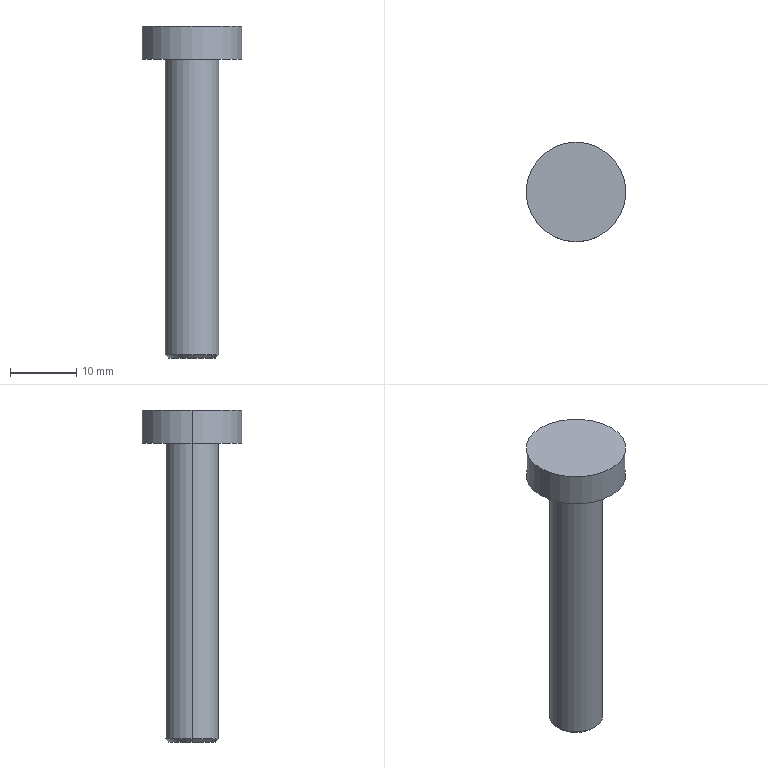Part | SolidWorks | features Chamfer 1, Extrusion 1, ICE 1 | 1 solid | 9 faces | box 15 x 15 x 50 mm | volume 3143 mm3 | cylinder 4 | plane 3 | cone 2 | commonest cylinder face diameters 8 x2 15 x2
STEP:
#1=CARTESIAN_POINT('',(-3.5,0.,0.));
#2=VERTEX_POINT('',#1);
#3=CARTESIAN_POINT('',(3.5,0.,0.));
#4=VERTEX_POINT('',#3);
#5=CARTESIAN_POINT('',(0.,0.,0.));
#6=DIRECTION('',(0.,0.,-1.));
#7=DIRECTION('',(1.,0.,0.));
#8=AXIS2_PLACEMENT_3D('',#5,#6,#7);
#9=CIRCLE('',#8,3.5);
#10=EDGE_CURVE('',#2,#4,#9,.T.);
#11=ORIENTED_EDGE('',*,*,#10,.F.);
#12=CARTESIAN_POINT('',(-4.,0.,0.5));
#13=VERTEX_POINT('',#12);
#14=CARTESIAN_POINT('',(-4.,0.,0.5));
#15=DIRECTION('',(-0.7071,0.,0.7071));
#16=VECTOR('',#15,1000.);
#17=LINE('',#14,#16);
#18=EDGE_CURVE('',#2,#13,#17,.T.);
#19=ORIENTED_EDGE('',*,*,#18,.T.);
#20=CARTESIAN_POINT('',(4.,0.,0.5));
#21=VERTEX_POINT('',#20);
#22=CARTESIAN_POINT('',(0.,0.,0.5));
#23=DIRECTION('',(0.,0.,1.));
#24=DIRECTION('',(1.,0.,0.));
#25=AXIS2_PLACEMENT_3D('',#22,#23,#24);
#26=CIRCLE('',#25,4.);
#27=EDGE_CURVE('',#21,#13,#26,.T.);
#28=ORIENTED_EDGE('',*,*,#27,.F.);
#29=CARTESIAN_POINT('',(4.,0.,0.5));
#30=DIRECTION('',(0.7071,0.,0.7071));
#31=VECTOR('',#30,1000.);
#32=LINE('',#29,#31);
#33=EDGE_CURVE('',#4,#21,#32,.T.);
#34=ORIENTED_EDGE('',*,*,#33,.F.);
#35=EDGE_LOOP('',(#11,#19,#28,#34));
#36=FACE_OUTER_BOUND('',#35,.T.);
#37=CARTESIAN_POINT('',(0.,0.,0.5));
#38=DIRECTION('',(0.,0.,1.));
#39=DIRECTION('',(1.,0.,0.));
#40=AXIS2_PLACEMENT_3D('',#37,#38,#39);
#41=CONICAL_SURFACE('',#40,4.,0.7854);
#42=ADVANCED_FACE('',(#36),#41,.T.);
#43=CARTESIAN_POINT('',(7.5,0.,50.));
#44=VERTEX_POINT('',#43);
#45=CARTESIAN_POINT('',(-7.5,0.,50.));
#46=VERTEX_POINT('',#45);
#47=CARTESIAN_POINT('',(0.,0.,50.));
#48=DIRECTION('',(0.,0.,1.));
#49=DIRECTION('',(1.,0.,0.));
#50=AXIS2_PLACEMENT_3D('',#47,#48,#49);
#51=CIRCLE('',#50,7.5);
#52=EDGE_CURVE('',#44,#46,#51,.T.);
#53=ORIENTED_EDGE('',*,*,#52,.F.);
#54=CARTESIAN_POINT('',(7.5,0.,45.));
#55=VERTEX_POINT('',#54);
#56=CARTESIAN_POINT('',(7.5,0.,50.));
#57=DIRECTION('',(0.,0.,-1.));
#58=VECTOR('',#57,1000.);
#59=LINE('',#56,#58);
#60=EDGE_CURVE('',#44,#55,#59,.T.);
#61=ORIENTED_EDGE('',*,*,#60,.T.);
#62=CARTESIAN_POINT('',(-7.5,0.,45.));
#63=VERTEX_POINT('',#62);
#64=CARTESIAN_POINT('',(0.,0.,45.));
#65=DIRECTION('',(0.,0.,1.));
#66=DIRECTION('',(1.,0.,0.));
#67=AXIS2_PLACEMENT_3D('',#64,#65,#66);
#68=CIRCLE('',#67,7.5);
#69=EDGE_CURVE('',#55,#63,#68,.T.);
#70=ORIENTED_EDGE('',*,*,#69,.T.);
#71=CARTESIAN_POINT('',(-7.5,0.,50.));
#72=DIRECTION('',(0.,0.,-1.));
#73=VECTOR('',#72,1000.);
#74=LINE('',#71,#73);
#75=EDGE_CURVE('',#46,#63,#74,.T.);
#76=ORIENTED_EDGE('',*,*,#75,.F.);
#77=EDGE_LOOP('',(#53,#61,#70,#76));
#78=FACE_OUTER_BOUND('',#77,.T.);
#79=CARTESIAN_POINT('',(0.,0.,50.));
#80=DIRECTION('',(0.,0.,-1.));
#81=DIRECTION('',(-1.,0.,0.));
#82=AXIS2_PLACEMENT_3D('',#79,#80,#81);
#83=CYLINDRICAL_SURFACE('',#82,7.5);
#84=ADVANCED_FACE('',(#78),#83,.T.);
#85=CARTESIAN_POINT('',(4.,0.,45.));
#86=VERTEX_POINT('',#85);
#87=CARTESIAN_POINT('',(-4.,0.,45.));
#88=VERTEX_POINT('',#87);
#89=CARTESIAN_POINT('',(0.,0.,45.));
#90=DIRECTION('',(0.,0.,1.));
#91=DIRECTION('',(1.,0.,0.));
#92=AXIS2_PLACEMENT_3D('',#89,#90,#91);
#93=CIRCLE('',#92,4.);
#94=EDGE_CURVE('',#86,#88,#93,.T.);
#95=ORIENTED_EDGE('',*,*,#94,.F.);
#96=CARTESIAN_POINT('',(4.,0.,45.));
#97=DIRECTION('',(0.,0.,-1.));
#98=VECTOR('',#97,1000.);
#99=LINE('',#96,#98);
#100=EDGE_CURVE('',#86,#21,#99,.T.);
#101=ORIENTED_EDGE('',*,*,#100,.T.);
#102=ORIENTED_EDGE('',*,*,#27,.T.);
#103=CARTESIAN_POINT('',(-4.,0.,45.));
#104=DIRECTION('',(0.,0.,-1.));
#105=VECTOR('',#104,1000.);
#106=LINE('',#103,#105);
#107=EDGE_CURVE('',#88,#13,#106,.T.);
#108=ORIENTED_EDGE('',*,*,#107,.F.);
#109=EDGE_LOOP('',(#95,#101,#102,#108));
#110=FACE_OUTER_BOUND('',#109,.T.);
#111=CARTESIAN_POINT('',(0.,0.,45.));
#112=DIRECTION('',(0.,0.,-1.));
#113=DIRECTION('',(-1.,0.,0.));
#114=AXIS2_PLACEMENT_3D('',#111,#112,#113);
#115=CYLINDRICAL_SURFACE('',#114,4.);
#116=ADVANCED_FACE('',(#110),#115,.T.);
#117=ORIENTED_EDGE('',*,*,#100,.F.);
#118=CARTESIAN_POINT('',(0.,0.,45.));
#119=DIRECTION('',(0.,0.,1.));
#120=DIRECTION('',(1.,0.,0.));
#121=AXIS2_PLACEMENT_3D('',#118,#119,#120);
#122=CIRCLE('',#121,4.);
#123=EDGE_CURVE('',#88,#86,#122,.T.);
#124=ORIENTED_EDGE('',*,*,#123,.F.);
#125=ORIENTED_EDGE('',*,*,#107,.T.);
#126=CARTESIAN_POINT('',(0.,0.,0.5));
#127=DIRECTION('',(0.,0.,1.));
#128=DIRECTION('',(1.,0.,0.));
#129=AXIS2_PLACEMENT_3D('',#126,#127,#128);
#130=CIRCLE('',#129,4.);
#131=EDGE_CURVE('',#13,#21,#130,.T.);
#132=ORIENTED_EDGE('',*,*,#131,.T.);
#133=EDGE_LOOP('',(#117,#124,#125,#132));
#134=FACE_OUTER_BOUND('',#133,.T.);
#135=CARTESIAN_POINT('',(0.,0.,45.));
#136=DIRECTION('',(0.,0.,-1.));
#137=DIRECTION('',(-1.,0.,0.));
#138=AXIS2_PLACEMENT_3D('',#135,#136,#137);
#139=CYLINDRICAL_SURFACE('',#138,4.);
#140=ADVANCED_FACE('',(#134),#139,.T.);
#141=CARTESIAN_POINT('',(0.,0.,0.));
#142=DIRECTION('',(0.,0.,-1.));
#143=DIRECTION('',(1.,0.,0.));
#144=AXIS2_PLACEMENT_3D('',#141,#142,#143);
#145=CIRCLE('',#144,3.5);
#146=EDGE_CURVE('',#4,#2,#145,.T.);
#147=ORIENTED_EDGE('',*,*,#146,.T.);
#148=ORIENTED_EDGE('',*,*,#10,.T.);
#149=EDGE_LOOP('',(#147,#148));
#150=FACE_OUTER_BOUND('',#149,.T.);
#151=CARTESIAN_POINT('',(0.,0.,0.));
#152=DIRECTION('',(0.,0.,1.));
#153=DIRECTION('',(1.,0.,0.));
#154=AXIS2_PLACEMENT_3D('',#151,#152,#153);
#155=PLANE('',#154);
#156=ADVANCED_FACE('',(#150),#155,.F.);
#157=CARTESIAN_POINT('',(0.,0.,45.));
#158=DIRECTION('',(0.,0.,1.));
#159=DIRECTION('',(1.,0.,0.));
#160=AXIS2_PLACEMENT_3D('',#157,#158,#159);
#161=CIRCLE('',#160,7.5);
#162=EDGE_CURVE('',#63,#55,#161,.T.);
#163=ORIENTED_EDGE('',*,*,#162,.F.);
#164=ORIENTED_EDGE('',*,*,#69,.F.);
#165=EDGE_LOOP('',(#163,#164));
#166=FACE_OUTER_BOUND('',#165,.T.);
#167=ORIENTED_EDGE('',*,*,#123,.T.);
#168=ORIENTED_EDGE('',*,*,#94,.T.);
#169=EDGE_LOOP('',(#167,#168));
#170=FACE_BOUND('',#169,.T.);
#171=CARTESIAN_POINT('',(0.,0.,45.));
#172=DIRECTION('',(0.,0.,1.));
#173=DIRECTION('',(1.,0.,0.));
#174=AXIS2_PLACEMENT_3D('',#171,#172,#173);
#175=PLANE('',#174);
#176=ADVANCED_FACE('',(#166,#170),#175,.F.);
#177=ORIENTED_EDGE('',*,*,#60,.F.);
#178=CARTESIAN_POINT('',(0.,0.,50.));
#179=DIRECTION('',(0.,0.,1.));
#180=DIRECTION('',(1.,0.,0.));
#181=AXIS2_PLACEMENT_3D('',#178,#179,#180);
#182=CIRCLE('',#181,7.5);
#183=EDGE_CURVE('',#46,#44,#182,.T.);
#184=ORIENTED_EDGE('',*,*,#183,.F.);
#185=ORIENTED_EDGE('',*,*,#75,.T.);
#186=ORIENTED_EDGE('',*,*,#162,.T.);
#187=EDGE_LOOP('',(#177,#184,#185,#186));
#188=FACE_OUTER_BOUND('',#187,.T.);
#189=CARTESIAN_POINT('',(0.,0.,50.));
#190=DIRECTION('',(0.,0.,-1.));
#191=DIRECTION('',(-1.,0.,0.));
#192=AXIS2_PLACEMENT_3D('',#189,#190,#191);
#193=CYLINDRICAL_SURFACE('',#192,7.5);
#194=ADVANCED_FACE('',(#188),#193,.T.);
#195=ORIENTED_EDGE('',*,*,#183,.T.);
#196=ORIENTED_EDGE('',*,*,#52,.T.);
#197=EDGE_LOOP('',(#195,#196));
#198=FACE_OUTER_BOUND('',#197,.T.);
#199=CARTESIAN_POINT('',(0.,0.,50.));
#200=DIRECTION('',(0.,0.,1.));
#201=DIRECTION('',(1.,0.,0.));
#202=AXIS2_PLACEMENT_3D('',#199,#200,#201);
#203=PLANE('',#202);
#204=ADVANCED_FACE('',(#198),#203,.T.);
#205=ORIENTED_EDGE('',*,*,#18,.F.);
#206=ORIENTED_EDGE('',*,*,#146,.F.);
#207=ORIENTED_EDGE('',*,*,#33,.T.);
#208=ORIENTED_EDGE('',*,*,#131,.F.);
#209=EDGE_LOOP('',(#205,#206,#207,#208));
#210=FACE_OUTER_BOUND('',#209,.T.);
#211=CARTESIAN_POINT('',(0.,0.,0.5));
#212=DIRECTION('',(0.,0.,1.));
#213=DIRECTION('',(1.,0.,0.));
#214=AXIS2_PLACEMENT_3D('',#211,#212,#213);
#215=CONICAL_SURFACE('',#214,4.,0.7854);
#216=ADVANCED_FACE('',(#210),#215,.T.);
#217=CLOSED_SHELL('',(#42,#84,#116,#140,#156,#176,#194,#204,#216));
#218=MANIFOLD_SOLID_BREP('',#217);
#219=CARTESIAN_POINT('',(0.,0.,0.));
#220=DIRECTION('',(0.,0.,1.));
#221=DIRECTION('',(1.,0.,0.));
#222=AXIS2_PLACEMENT_3D('',#219,#220,#221);
#223=(LENGTH_UNIT()NAMED_UNIT(*)SI_UNIT(.MILLI.,.METRE.));
#224=UNCERTAINTY_MEASURE_WITH_UNIT(LENGTH_MEASURE(0.00001),#223,'','');
#225=(NAMED_UNIT(*)PLANE_ANGLE_UNIT()SI_UNIT($,.RADIAN.));
#226=(NAMED_UNIT(*)SI_UNIT($,.STERADIAN.)SOLID_ANGLE_UNIT());
#227=(GEOMETRIC_REPRESENTATION_CONTEXT(3)GLOBAL_UNCERTAINTY_ASSIGNED_CONTEXT((#224))GLOBAL_UNIT_ASSIGNED_CONTEXT((#223,#225,#226))REPRESENTATION_CONTEXT('',''));
#228=ADVANCED_BREP_SHAPE_REPRESENTATION('',(#218,#222),#227);